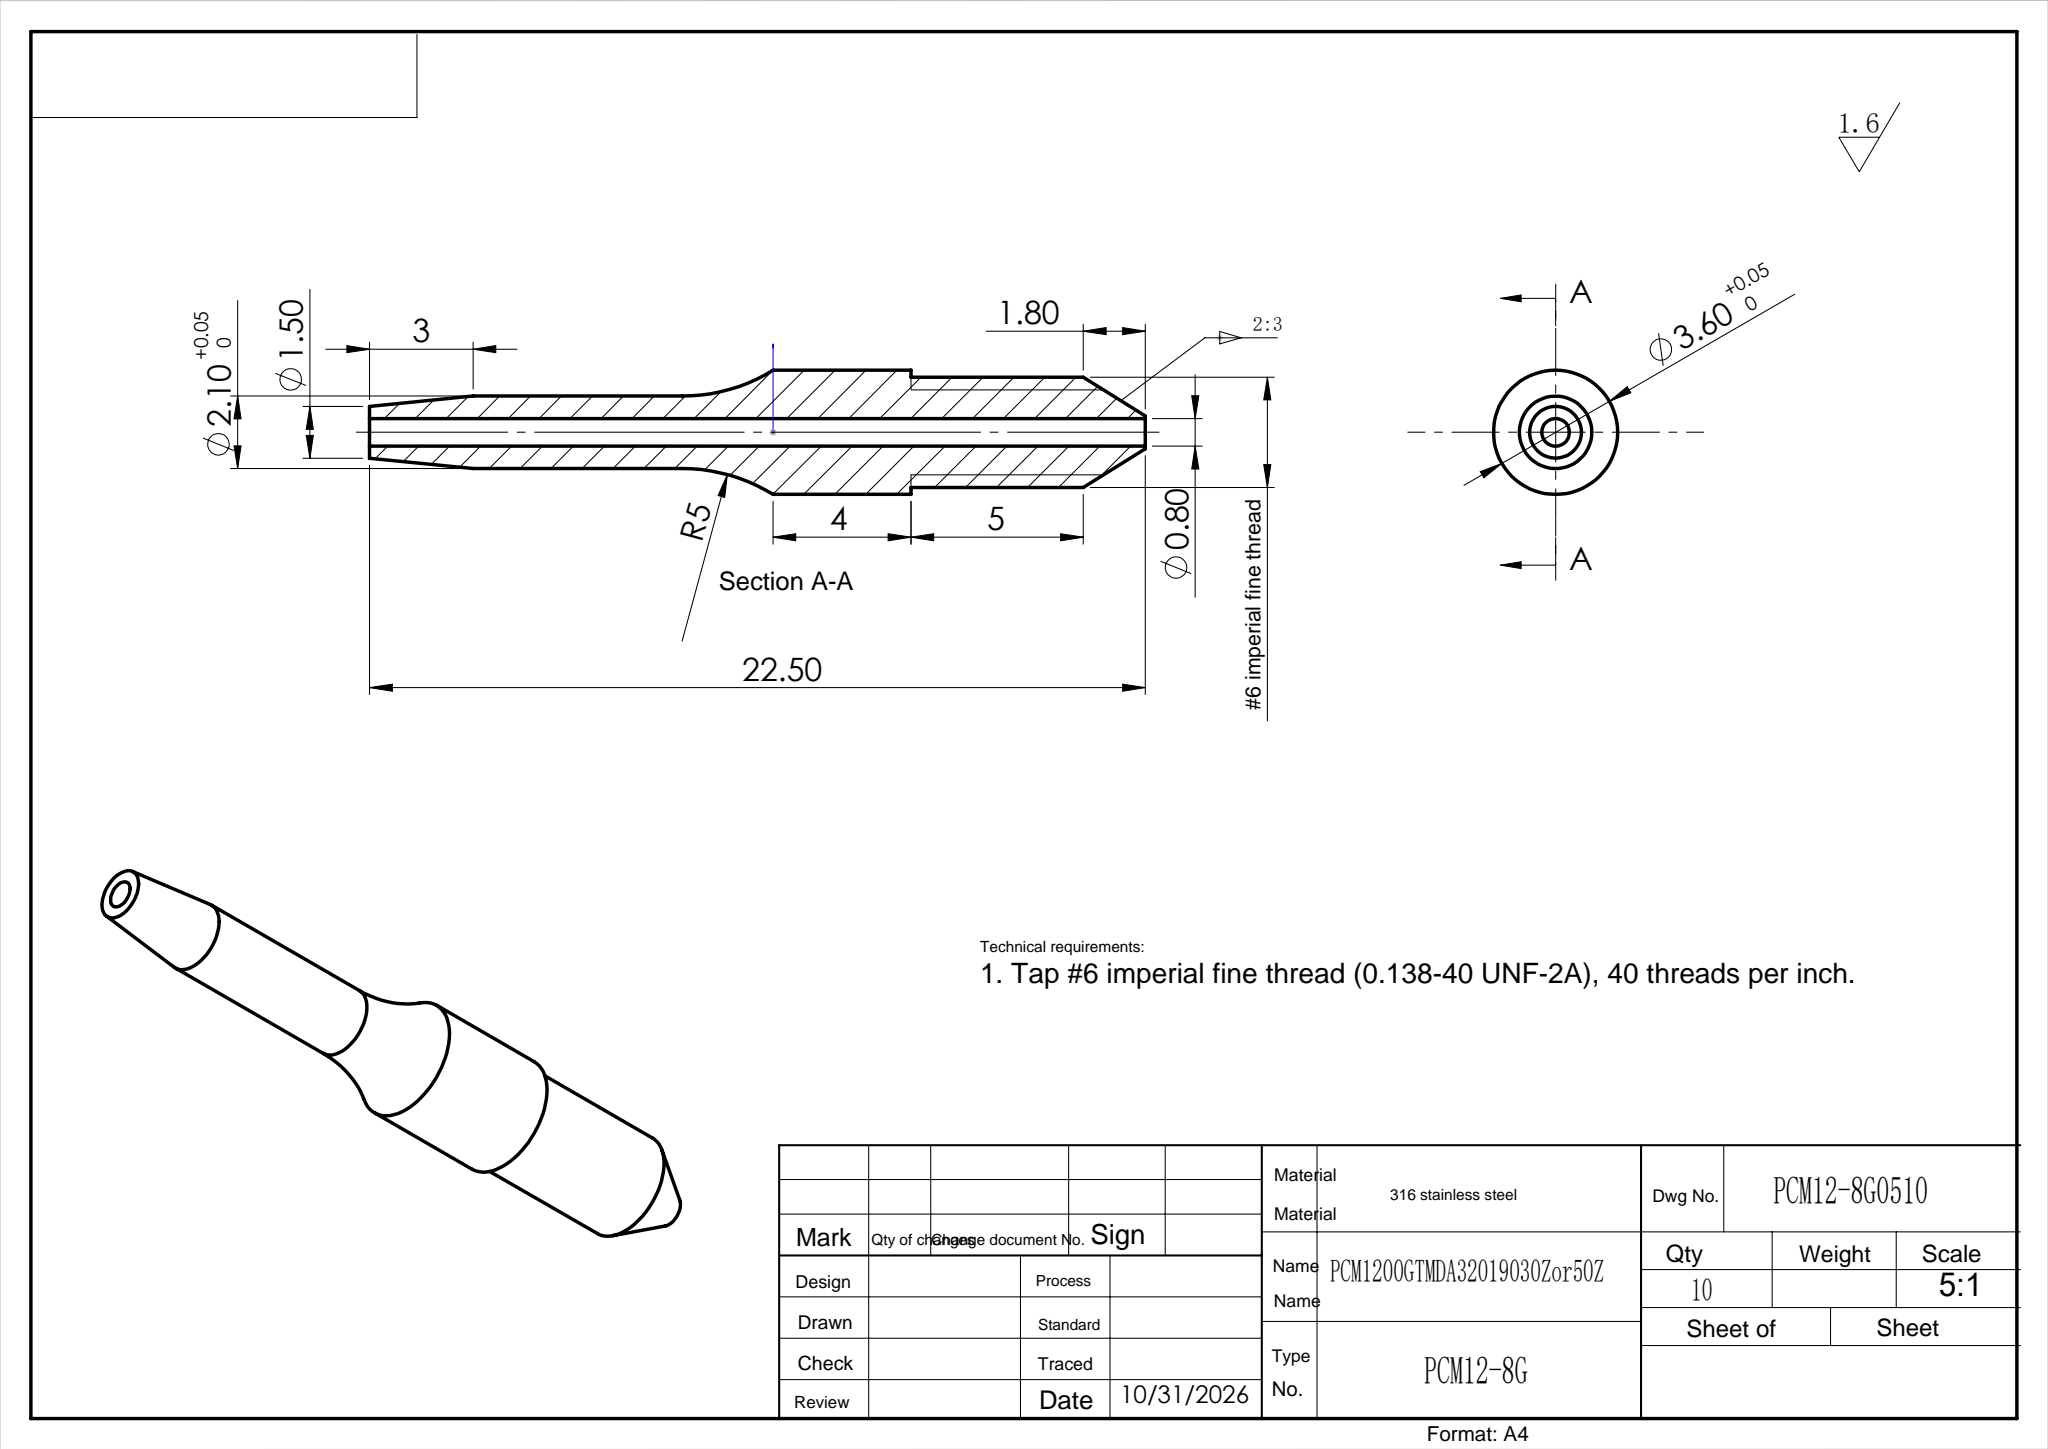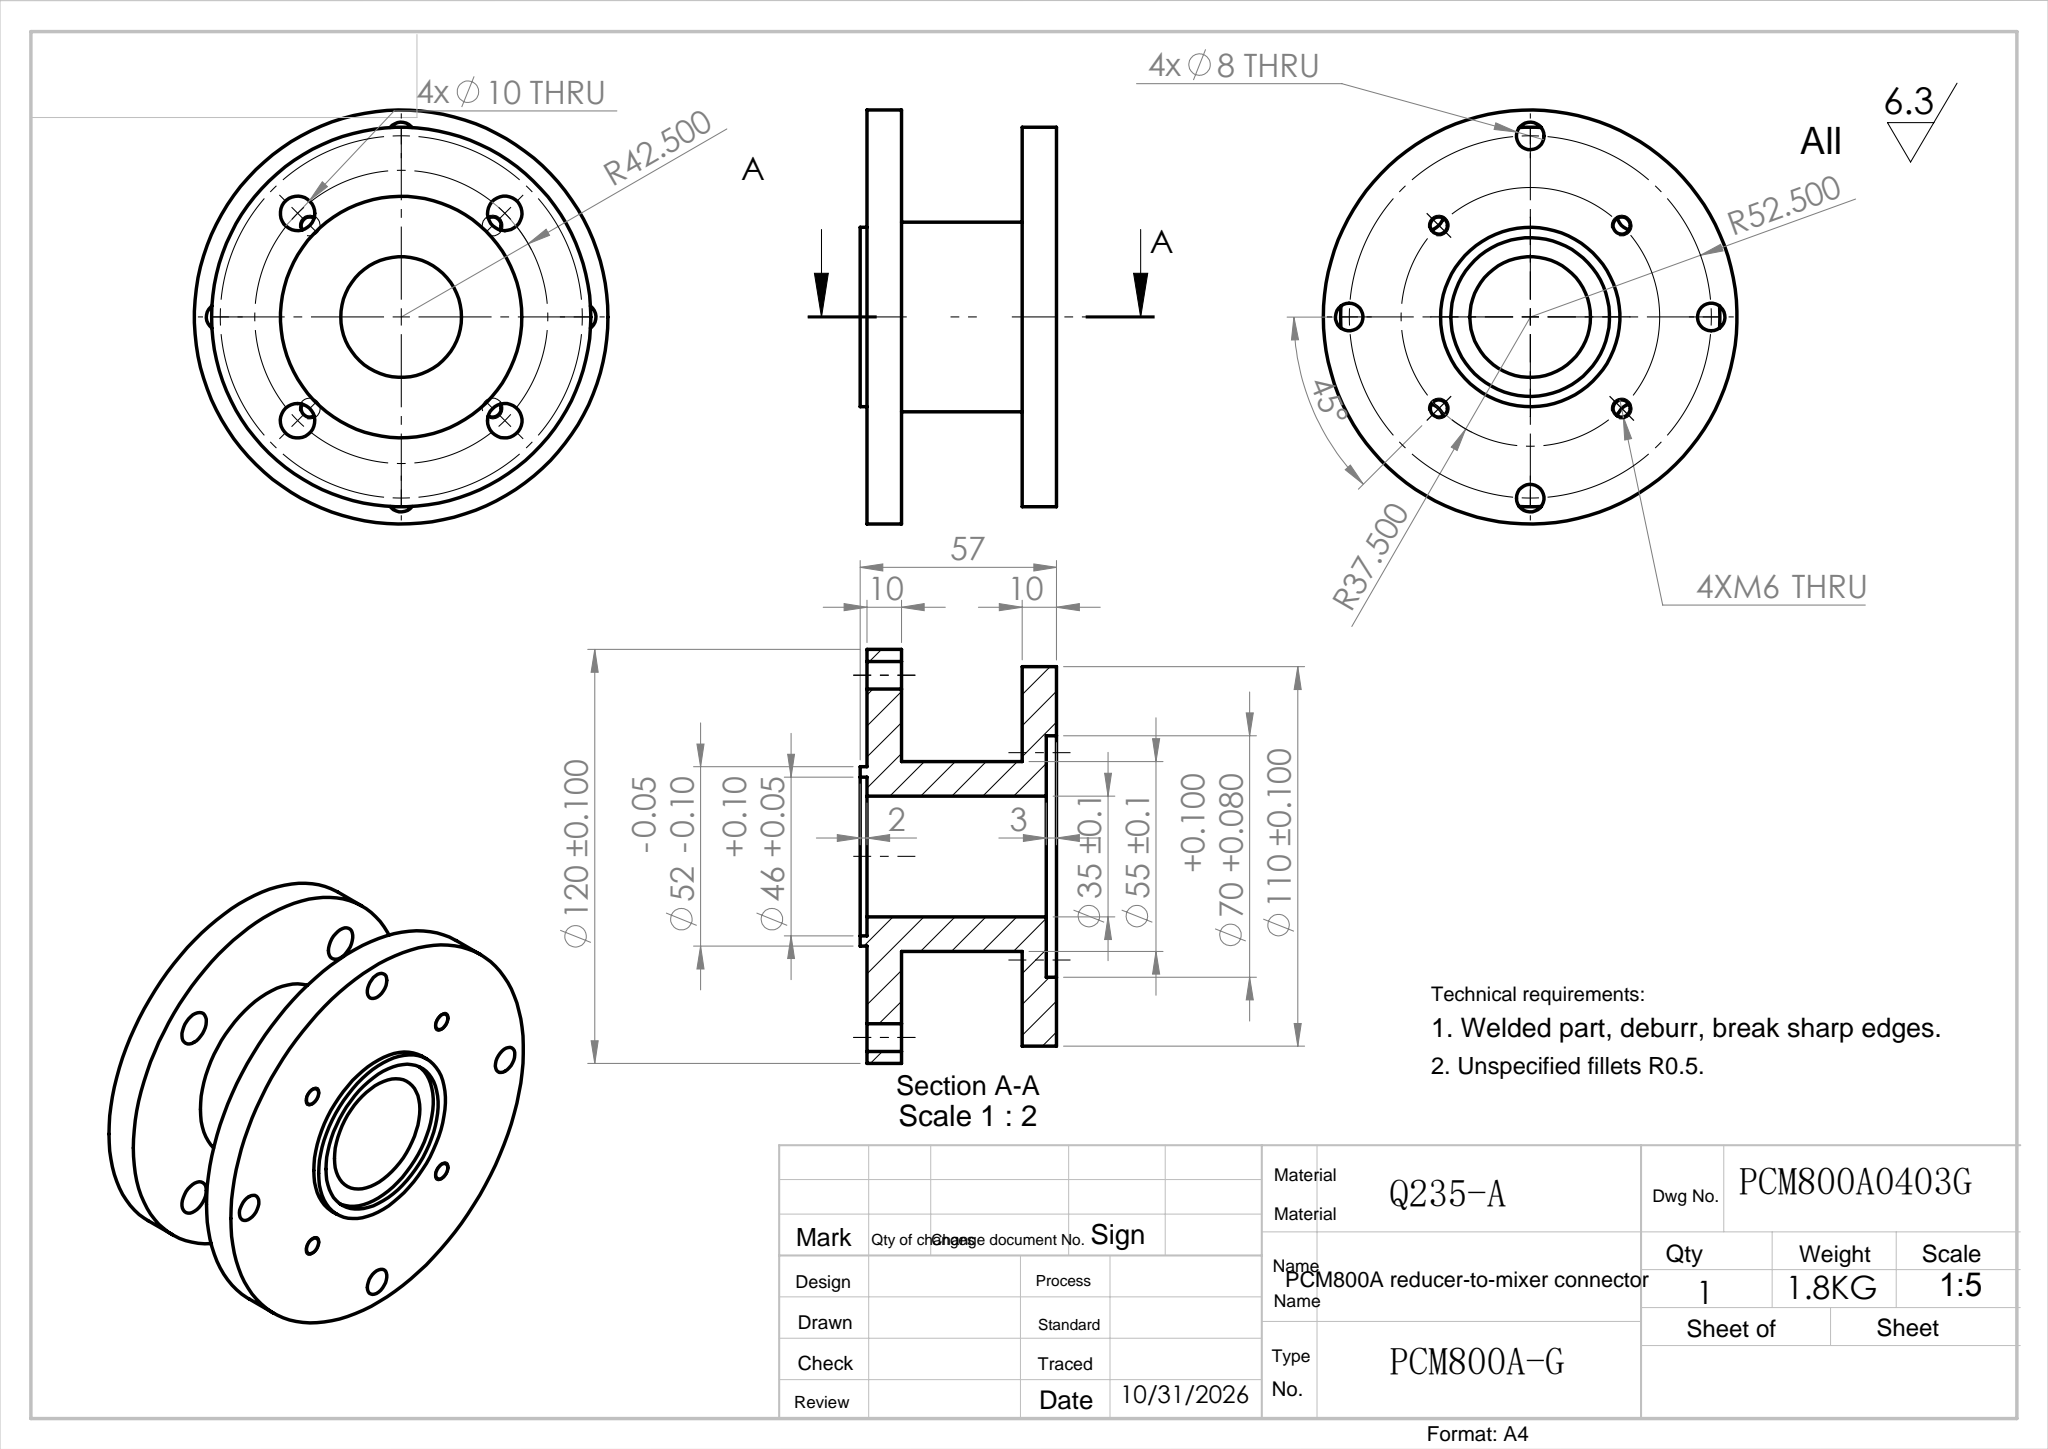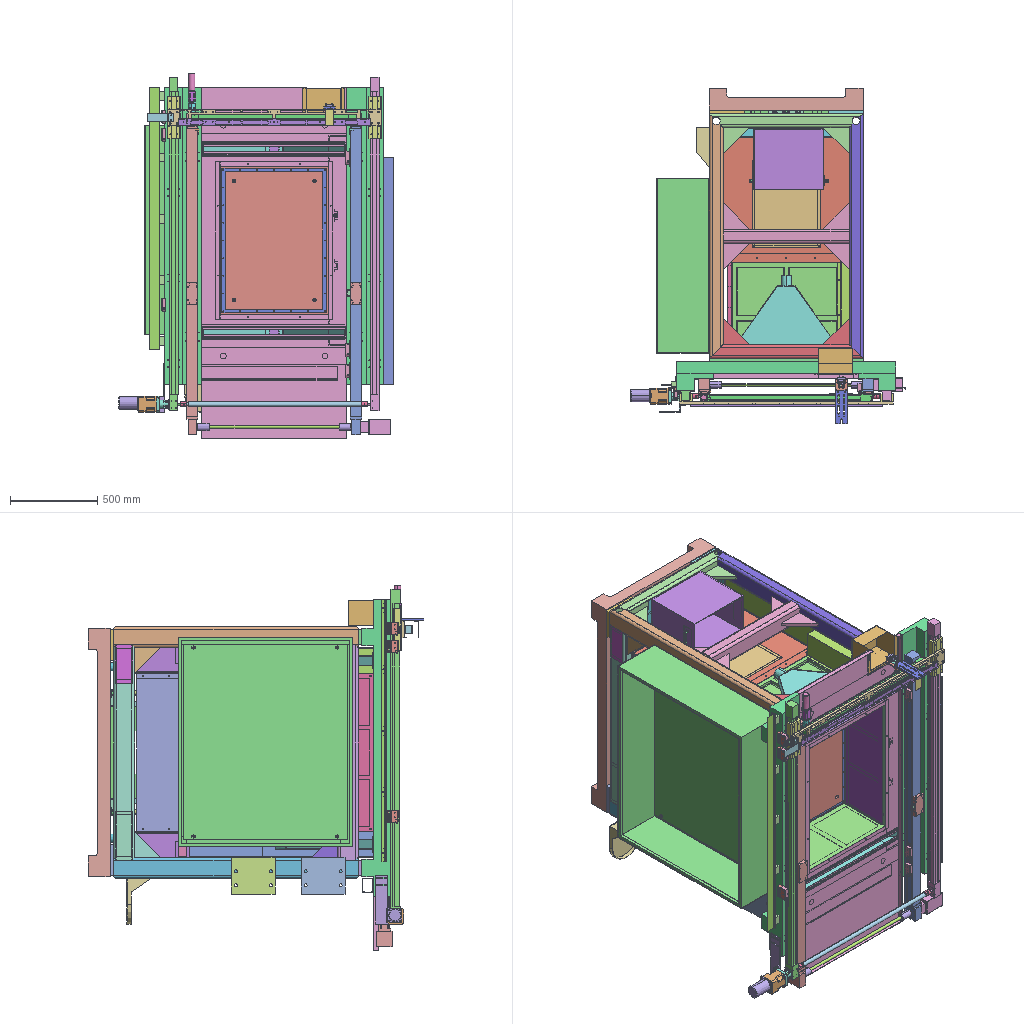Assembly | SolidWorks | 213 different items | 390 placed | box 1571 x 1918 x 2089 mm
Parts list (item | name | quantity | parent item | size | volume | features):
1 | (subassembly) | x1 | in 20 | 45.671 x 31.209 x 79.324 mm | 36091 mm3 | -
2 | (subassembly) | x2 | in 1 | 11.2 x 79.113 x 5.6 mm | 906.583 mm3 | features CompositeCurve 1
3 | (subassembly) | x1 | in 20 | 158.75 x 253.079 x 184.571 mm | 227945 mm3 | -
4 | (subassembly) | x2 | in 6 | 450 x 350 x 250 mm | 2820249 mm3 | features AEMSimFeature 1
5 | (subassembly) | x2 | in 8 | 202.5 x 1859 x 119.5 mm | 4220516 mm3 | features CompositeCurve 1
6 | (subassembly) | x1 | - | 1731 x 1422 x 2008 mm | 170873319 mm3 | features CompositeCurve 1
7 | (subassembly) | x1 | - | - | 100167004 mm3 | features ReferencePattern 16, CompositeCurve 9, LocalLPattern 2
8 | (subassembly) | x1 | - | - | 140729091 mm3 | features CompositeCurve 2
9 | (subassembly) | x2 | in 7 | 121 x 153.5 x 29.5 mm | 51392 mm3 | -
10 | (subassembly) | x2 | in 7 | 52.5 x 15 x 65 mm | 16522 mm3 | -
11 | (subassembly) | x1 | in 7 | 103 x 363 x 86 mm | 1173870 mm3 | -
12 | (subassembly) | x1 | in 7 | 64.002 x 64.002 x 160 mm | 203839 mm3 | -
13 | (subassembly) | x1 | in 7 | 45.805 x 40.368 x 35 mm | 17683 mm3 | -
14 | (subassembly) | x3 | - | 26 x 65 x 74.506 mm | 84061 mm3 | -
15 | (subassembly) | x3 | - | 100 x 42 x 26 mm | 68056 mm3 | -
16 | (subassembly) | x2 | in 7 | 120 x 42 x 41 mm | 79565 mm3 | -
17 | (subassembly) | x1 | in 8 | 700 x 1398 x 750 mm | 37335831 mm3 | features AEMSimFeature 1
18 | (subassembly) | x1 | - | 1167 x 88 x 1837 mm | 15808728 mm3 | -
19 | (subassembly) | x1 | in 17 | 472.19 x 352.538 x 235.211 mm | 7182982 mm3 | features AEMSimFeature 1
20 | (subassembly) | x1 | - | 300.5 x 279.222 x 1337 mm | 3097922 mm3 | features CompositeCurve 1
21 | (subassembly) | x1 | - | 2273 x 1295 x 1895 mm | 10477975 mm3 | -
22 | - | x1 | in 8 | 782 x 83 x 1038 mm | 2557655 mm3 | features ICE 6, Extrusion 1, Shell 1
23 | - | x2 | in 2 | 3.4 x 3.4 x 17.8 mm | 96.571 mm3 | features Boss 2, Chamfer 1, Cut 1, Extrusion 1, Fillet 1
24 | - | x2 | in 2 | 3.6 x 3.6 x 17.8 mm | 95.144 mm3 | features Chamfer 3, Boss 2, Extrusion 1
25 | - | x2 | in 2 | 5.6 x 11.2 x 40 mm | 624.39 mm3 | features Boss 6, Cut 3, Fillet 3, MirrorPattern 3, Chamfer 1, Extrusion 1, Sweep 1
26 | - | x1 | in 1 | 15 x 18 x 30 mm | 6618 mm3 | features Cut 3, Extrusion 1, LPattern 1
27 | - | x1 | in 1 | 12.5 x 8 x 8.081 mm | 341.66 mm3 | features Boss 1, Cut 1, Extrusion 1
28 | - | x1 | in 1 | 35 x 24 x 45 mm | 15822 mm3 | features Cut 6, Boss 2, MirrorPattern 2, Extrusion 1, Fillet 1
29 | - | x1 | in 1 | 55 x 12.5 x 40 mm | 11308 mm3 | features Boss 3, Cut 3, Extrusion 1, Fillet 1, HoleWzd 1, ICE 1, MirrorPattern 1
30 | - | x1 | in 3 | 72 x 66 x 80 mm | 80733 mm3 | features Boss 3, HoleWzd 3, Extrusion 1, MirrorPattern 1
31 | - | x1 | in 3 | 66 x 10 x 190 mm | 102125 mm3 | features Cut 2, HoleWzd 2, Extrusion 1
32 | - | x1 | in 3 | 51 x 261 x 69 mm | 43977 mm3 | features Extrusion 1, ICE 1, LPattern 1, Shell 1
33 | - | x1 | in 8 | 841 x 100 x 1142 mm | 2713356 mm3 | features ICE 5, Extrusion 1, Shell 1
34 | - | x2 | in 2 | 3 x 3 x 20 mm | 90.478 mm3 | features Extrusion 1
35 | - | x1 | in 6 | 280 x 70 x 48.5 mm | 177998 mm3 | features Extrusion 1, HoleWzd 1, ICE 1
36 | - | x1 | in 6 | 78.5 x 60 x 800 mm | 272371 mm3 | features ExtruThin 1, HoleWzd 1, MirrorPattern 1
37 | - | x1 | in 6 | 8 x 63 x 800 mm | 91142 mm3 | features ExtruThin 1, HoleWzd 1, MirrorPattern 1
38 | - | x1 | in 6 | 238 x 166 x 150 mm | 256776 mm3 | features ICE 2, Extrusion 1, Shell 1
39 | - | x2 | in 6 | 822.906 x 560 x 70 mm | 1097243 mm3 | features ICE 2, Extrusion 1, Shell 1
40 | - | x2 | in 4 | 410 x 350 x 250 mm | 2798000 mm3 | features ICE 2, Extrusion 1, Shell 1
41 | - | x4 | in 4 | 120 x 20 x 15 mm | 11124 mm3 | features Extrusion 1, Fillet 1, ICE 1
42 | - | x2 | in 6 | 715 x 153 x 250 mm | 795621 mm3 | features ICE 5, Extrusion 1
43 | - | x1 | in 8 | 295 x 2005 x 250 mm | 2083546 mm3 | features ICE 7, Extrusion 1, Shell 1
44 | - | x2 | in 5 | 202.5 x 359 x 119.5 mm | 3868562 mm3 | features ICE 6, Extrusion 1
45 | - | x1 | in 6 | 880 x 125 x 1420 mm | 55146557 mm3 | features Fillet 3, 3DProfileFeature 2, Cut 2, HoleWzd 2, LPattern 2, Extrusion 1, ICE 1
46 | - | x1 | in 6 | 220 x 100 x 1 mm | 22000 mm3 | features Extrusion 1
47 | - | x1 | in 6 | 280 x 100 x 1 mm | 28000 mm3 | features Extrusion 1
48 | - | x1 | in 6 | 60 x 60 x 1 mm | 2477 mm3 | features Extrusion 1
49 | - | x1 | in 6 | 55 x 11 x 55 mm | 19851 mm3 | features Revolution 1
50 | - | x1 | - | 146 x 1366 x 130.5 mm | 474775 mm3 | features ICE 8, HoleWzd 2, Extrusion 1
51 | - | x1 | in 8 | 150 x 480 x 2005 mm | 2840339 mm3 | features ICE 8, ExtruThin 1
52 | - | x1 | - | 146 x 1366 x 130.5 mm | 474775 mm3 | features ICE 8, HoleWzd 2, Extrusion 1
53 | - | x1 | in 6 | 1438 x 898.415 x 1530 mm | 49681845 mm3 | features ICE 6, Boss 5, MirrorPattern 4, WeldMemberFeat 3, HoleWzd 2, LPattern 2, MirrorSolid 2, 3DProfileFeature 1, Cut 1, WeldmentFeature 1
54 | - | x1 | in 6 | 120 x 60 x 50 mm | 42021 mm3 | features ExtruThin 1, ICE 1
55 | - | x1 | in 6 | 1200 x 1000 x 300 mm | 7626457 mm3 | features ICE 7, LPattern 3, Extrusion 1, Fillet 1, Shell 1
56 | - | x1 | in 6 | 230 x 250 x 265 mm | 373785 mm3 | features ICE 4, Rib 2, Extrusion 1
57 | - | x1 | in 6 | 830 x 2008 x 32.5 mm | 2572177 mm3 | features ICE 8, Extrusion 1, LPattern 1
58 | - | x1 | in 6 | 1252 x 168 x 1700 mm | 44599924 mm3 | features ICE 4, HoleWzd 3, Fillet 2, Shell 2, Extrusion 1, MirrorPattern 1
59 | - | x2 | in 5 | 76 x 76 x 1500 mm | 351954 mm3 | features Extrusion 1, ICE 1
60 | - | x1 | in 8 | 787 x 165 x 100 mm | 713791 mm3 | features ICE 2, Extrusion 1, Shell 1
61 | - | x4 | in 7 | 110 x 10 x 110 mm | 48026 mm3 | features HoleWzd 1, Revolution 1
62 | - | x2 | in 7 | 623 x 635 x 25 mm | 3690263 mm3 | features Boss 8, Cut 3, 3DProfileFeature 2, HoleWzd 2, Chamfer 1, Extrusion 1, Fillet 1
63 | - | x2 | in 7 | 25 x 635 x 2 mm | 31411 mm3 | features Cut 1, Extrusion 1, LPattern 1
64 | - | x2 | in 7 | 47 x 14 x 47 mm | 19838 mm3 | features Chamfer 1, Extrusion 1
65 | - | x2 | in 7 | 110 x 110 x 24 mm | 185226 mm3 | features Cut 3, 3DProfileFeature 2, Chamfer 2, HoleWzd 2, Extrusion 1, Fillet 1
66 | - | x2 | in 7 | 75 x 10 x 75 mm | 20954 mm3 | features Chamfer 2, Boss 1, Cut 1, Extrusion 1, Fillet 1
67 | - | x8 | in 7 | 23 x 115 x 10 mm | 9831 mm3 | features Extrusion 1, ICE 1
68 | - | x2 | in 7 | 47 x 44 x 47 mm | 38423 mm3 | features Boss 2, Chamfer 1, Cut 1, Extrusion 1
69 | - | x2 | in 7 | 200 x 79 x 115 mm | 1064261 mm3 | features Cut 7, Boss 2, HoleWzd 2, ICE 2, Extrusion 1, Fillet 1, MirrorPattern 1
70 | - | x2 | in 7 | 186.408 x 27 x 186.408 mm | 546884 mm3 | features Cut 5, Chamfer 3, Extrusion 1
71 | - | x1 | in 8 | 1204 x 492 x 30 mm | 1446455 mm3 | features ICE 3, Extrusion 1, Shell 1
72 | - | x4 | in 7 | 760 x 29 x 34 mm | 720073 mm3 | features Cut 2, Extrusion 1, LPattern 1
73 | - | x20 | in 7 | 23 x 20 x 9 mm | 3318 mm3 | features Cut 2, Extrusion 1
74 | - | x4 | in 7 | 135 x 40.5 x 70 mm | 280823 mm3 | features Cut 2, Extrusion 1
75 | - | x4 | in 7 | 50 x 50 x 835 mm | 1540803 mm3 | features Boss 2, Extrusion 1, HoleWzd 1, ICE 1, RevCut 1
76 | - | x8 | in 7 | 49.742 x 49.742 x 8 mm | 7088 mm3 | features Extrusion 1
77 | - | x1 | in 7 | 740 x 870 x 540 mm | 47222068 mm3 | features HoleWzd 9, 3DProfileFeature 8, MirrorPattern 7, Cut 5, Fillet 5, Boss 2, LPattern 2, Extrusion 1
78 | - | x3 | in 7 | 10.158 x 8.5 x 585 mm | 43311 mm3 | features Extrusion 1
79 | - | x2 | in 7 | 25 x 834 x 25 mm | 365070 mm3 | features Boss 4, Fillet 2, Chamfer 1, Extrusion 1
80 | - | x2 | in 7 | 48 x 81 x 62 mm | 73064 mm3 | features Boss 2, Cut 2, Chamfer 1, Extrusion 1
81 | - | x2 | in 7 | 520 x 100 x 100 mm | 2650054 mm3 | features Cut 5, Attribute 4, ICE 3, Extrusion 1, Fillet 1, HoleWzd 1, MirrorPattern 1
82 | - | x1 | in 8 | 1204 x 230 x 30 mm | 710869 mm3 | features ICE 3, Extrusion 1, Shell 1
83 | - | x4 | in 7 | 47 x 15 x 47 mm | 22564 mm3 | features Extrusion 1, Fillet 1
84 | - | x2 | in 7 | 80 x 80 x 17 mm | 23688 mm3 | features Boss 2, Chamfer 1, Cut 1, Extrusion 1, Fillet 1
85 | - | x2 | in 7 | 28 x 16 x 28 mm | 5744 mm3 | features Chamfer 1, Extrusion 1
86 | - | x2 | in 7 | 37 x 18 x 37 mm | 13677 mm3 | features Fillet 3, HoleWzd 3, 3DProfileFeature 2, Boss 1, CirPattern 1, Cut 1, Extrusion 1, ICE 1
87 | - | x2 | in 7 | 90 x 75 x 12 mm | 42464 mm3 | features Cut 2, Boss 1, Extrusion 1
88 | - | x1 | in 7 | 900 x 760 x 50 mm | 1252591 mm3 | features ICE 4, Cut 2, HoleWzd 2, Extrusion 1, Fillet 1, MirrorPattern 1, Shell 1
89 | - | x2 | in 7 | 390 x 500 x 1 mm | 194905 mm3 | features Extrusion 1, ICE 1
90 | - | x2 | in 7 | 760 x 720 x 30 mm | 624524 mm3 | features ICE 7, Fillet 2, Extrusion 1, HoleWzd 1
91 | - | x2 | in 7 | 903 x 720 x 1 mm | 649804 mm3 | features Extrusion 1, ICE 1
92 | - | x1 | in 7 | 827 x 5 x 597 mm | 274573 mm3 | features LPattern 3, Cut 1, Extrusion 1
93 | - | x2 | in 8 | 598.5 x 1319 x 28 mm | 1912739 mm3 | features Extrusion 1, ICE 1, Shell 1
94 | - | x1 | in 7 | 60 x 635 x 900 mm | 5489881 mm3 | features Boss 5, 3DProfileFeature 2, HoleWzd 2, Extrusion 1, MirrorPattern 1
95 | - | x1 | in 7 | 60 x 25 x 900 mm | 665333 mm3 | features 3DProfileFeature 3, HoleWzd 3, Boss 1, Chamfer 1, Cut 1, Extrusion 1, LPattern 1
96 | - | x1 | in 7 | 25 x 900 x 25 mm | 491836 mm3 | features 3DProfileFeature 2, HoleWzd 2, Chamfer 1, Cut 1, Extrusion 1, LPattern 1
97 | - | x1 | in 7 | 25 x 583 x 900 mm | 4907028 mm3 | features Boss 4, 3DProfileFeature 3, HoleWzd 3, LPattern 3, Chamfer 2, Cut 2, Extrusion 1
98 | - | x2 | in 9 | 95 x 20 x 120 mm | 16175 mm3 | features ICE 2, Chamfer 1, Extrusion 1
99 | - | x2 | in 9 | 72 x 29.5 x 20 mm | 17819 mm3 | features Extrusion 1, Fillet 1, ICE 1
100 | - | x2 | in 7 | 200 x 55 x 20 mm | 28430 mm3 | features ExtruThin 1, ICE 1
101 | - | x2 | in 10 | 35 x 65 x 10 mm | 6719 mm3 | features Fillet 1, Sweep 1
102 | - | x2 | in 9 | 70 x 130 x 23.5 mm | 17397 mm3 | features ICE 2, Extrusion 1, LPattern 1
103 | - | x4 | in 10 | 45 x 13 x 20 mm | 4902 mm3 | features Extrusion 1, Fillet 1, ICE 1
104 | - | x1 | in 8 | 1210 x 260 x 30 mm | 849119 mm3 | features ICE 3, Extrusion 1, Shell 1
105 | - | x1 | in 7 | 617 x 20 x 847 mm | 9301034 mm3 | features LPattern 3, Cut 2, HoleWzd 2, ICE 2, 3DProfileFeature 1, Extrusion 1
106 | - | x1 | in 7 | 10.158 x 8.5 x 900 mm | 66632 mm3 | features Extrusion 1
107 | - | x1 | in 11 | 124 x 13 x 13 mm | 14963 mm3 | features Boss 6, Fillet 3, Chamfer 1, Cut 1
108 | - | x1 | in 11 | 102.5 x 50 x 85 mm | 153933 mm3 | features Cut 3, 3DProfileFeature 1, Boss 1, Extrusion 1, HoleWzd 1, Split 1, WeldBeadFeat 1, WeldmentFeature 1
109 | - | x1 | in 11 | 80 x 80 x 184 mm | 810663 mm3 | features ICE 6, CombineBodies 1, Extrusion 1, Fillet 1
110 | - | x1 | in 11 | 103 x 53 x 86 mm | 69237 mm3 | features HoleWzd 2, 3DProfileFeature 1, Boss 1, Extrusion 1, ICE 1, Split 1, WeldBeadFeat 1, WeldmentFeature 1
111 | - | x1 | in 11 | 50 x 78 x 38 mm | 42138 mm3 | features Cut 3, Chamfer 2, Gusset 2, WeldBeadFeat 2, Boss 1, Extrusion 1, Fillet 1, WeldmentFeature 1
112 | - | x1 | in 8 | 1210 x 230 x 30 mm | 714301 mm3 | features ICE 3, Extrusion 1, Shell 1
113 | - | x1 | in 11 | 38 x 30 x 38 mm | 16522 mm3 | features Boss 2, Extrusion 1
114 | - | x1 | in 11 | 35.736 x 27 x 35.736 mm | 11879 mm3 | features Cut 2, Chamfer 1, Extrusion 1
115 | - | x1 | in 11 | 25 x 4 x 4 mm | 393.133 mm3 | features Extrusion 1
116 | - | x1 | in 11 | 40 x 40 x 66 mm | 50078 mm3 | features Cut 5, Boss 2, Chamfer 1, Extrusion 1
117 | - | x2 | in 11 | 24 x 6 x 24 mm | 2031 mm3 | features Chamfer 1, Extrusion 1
118 | - | x2 | in 12, 13 | 40 x 40 x 100 mm | 62655 mm3 | features Fillet 1, MirrorStock 1
119 | - | x1 | in 12 | 50 x 49 x 49 mm | 86970 mm3 | features HoleWzd 2, Extrusion 1, ICE 1
120 | - | x4 | in 12, 13 | 19 x 1.5 x 19 mm | 138.591 mm3 | features Extrusion 1
121 | - | x1 | in 13 | 50 x 49 x 49 mm | 86970 mm3 | features HoleWzd 2, Extrusion 1, ICE 1
122 | - | x4 | in 12, 13 | 35 x 11 x 35 mm | 8600 mm3 | features MirrorStock 1
123 | - | x2 | in 8 | 1346 x 22 x 288 mm | 1655952 mm3 | features ICE 2, Extrusion 1, Shell 1
124 | - | x1 | in 8 | 641 x 270 x 2005 mm | 4371242 mm3 | features ICE 11, ExtruThin 1
125 | - | x2 | in 12, 13 | 49 x 10 x 49 mm | 22243 mm3 | features 3DProfileFeature 1, Cut 1, Extrusion 1, HoleWzd 1
126 | - | x4 | in 12, 13 | 1 x 19.276 x 18.3 mm | 102.745 mm3 | features Boss 1, Cut 1, Extrusion 1
127 | - | x2 | in 12, 13 | 15 x 48 x 15 mm | 8443 mm3 | features MirrorStock 1
128 | - | x2 | in 12, 13 | 12 x 12 x 61 mm | 5846 mm3 | features ICE 3, Chamfer 2, MirrorStock 1
129 | - | x2 | in 7 | 70 x 30 x 10.5 mm | 20714 mm3 | features Extrusion 1
130 | - | x8 | in 14, 15, 16 | 74.506 x 42 x 21 mm | 49715 mm3 | features Extrusion 1, ICE 1
131 | - | x3 | in 15 | 100 x 37 x 5 mm | 18341 mm3 | features Extrusion 1, ICE 1
132 | - | x3 | in 14 | 20 x 60 x 70 mm | 34346 mm3 | features ICE 2, Extrusion 1
133 | - | x2 | in 16 | 120 x 37 x 5 mm | 21137 mm3 | features Extrusion 1
134 | - | x4 | in 16 | 20 x 20 x 15 mm | 4356 mm3 | features Extrusion 1
135 | - | x1 | in 8 | 370 x 270 x 2005 mm | 2609209 mm3 | features ICE 10, ExtruThin 1
136 | - | x2 | - | 40 x 25 x 12 mm | 6861 mm3 | features ICE 2, Extrusion 1, Fillet 1
137 | - | x1 | in 7 | 70 x 36 x 15 mm | 19658 mm3 | features Extrusion 1, Fillet 1, HoleWzd 1
138 | - | x2 | in 8 | 601 x 1551 x 28 mm | 2239470 mm3 | features Extrusion 1, ICE 1, Shell 1
139 | - | x1 | in 8 | 645 x 596 x 22 mm | 953984 mm3 | features Extrusion 1, ICE 1, Shell 1
140 | - | x1 | in 8 | 1457 x 492 x 30 mm | 1732596 mm3 | features ICE 3, Extrusion 1, Shell 1
141 | - | x2 | - | 128 x 64 x 20 mm | 161397 mm3 | features HoleWzd 2, MirrorPattern 2, Extrusion 1, LPattern 1
142 | - | x1 | in 18 | 72 x 88 x 1836 mm | 7220915 mm3 | features Boss 5, Cut 2, Extrusion 1, MirrorPattern 1
143 | - | x1 | in 8 | 1457 x 230 x 30 mm | 855585 mm3 | features ICE 3, Extrusion 1, Shell 1
144 | - | x1 | in 18 | 80 x 88 x 1836 mm | 7212179 mm3 | features Boss 5, Cut 2, MirrorPattern 2, Extrusion 1
145 | - | x1 | in 18 | 90 x 80 x 175 mm | 1069126 mm3 | features Boss 1, Chamfer 1, Cut 1, Extrusion 1
146 | - | x1 | in 18 | 16 x 16 x 770 mm | 154818 mm3 | features Extrusion 1
147 | - | x1 | in 6 | 55.5 x 21 x 1300 mm | 146072 mm3 | features ExtruThin 1, ICE 1
148 | - | x2 | in 18 | 40 x 40 x 67 mm | 70724 mm3 | features Extrusion 1, ICE 1
149 | - | x1 | in 18 | 35 x 32 x 20 mm | 5122 mm3 | features ICE 2, Extrusion 1
150 | - | x1 | in 18 | 35 x 32 x 20 mm | 5122 mm3 | features ICE 2, Extrusion 1
151 | - | x2 | in 8 | 724.5 x 1319 x 28 mm | 2267303 mm3 | features Extrusion 1, ICE 1, Shell 1
152 | - | x1 | in 8 | 2010 x 1894 x 432 mm | 6181114 mm3 | features ICE 6, WeldMemberFeat 3, WeldmentFeature 1
153 | - | x1 | in 8 | 2010 x 1894 x 230 mm | 4743265 mm3 | features ICE 6, WeldMemberFeat 3, WeldmentFeature 1
154 | - | x1 | in 8 | 841 x 100 x 658 mm | 1673891 mm3 | features ICE 5, Extrusion 1, Shell 1
155 | - | x1 | in 8 | 1740 x 2160 x 55 mm | 4890635 mm3 | features ICE 7, WeldMemberFeat 1, WeldmentFeature 1
156 | - | x1 | in 8 | 745 x 1196 x 22 mm | 2073584 mm3 | features Extrusion 1, ICE 1, Shell 1
157 | - | x1 | in 8 | 980 x 650 x 1400 mm | 5357860 mm3 | features ICE 6, Extrusion 1
158 | - | x1 | in 8 | 980 x 100 x 1400 mm | 3675222 mm3 | features ICE 8, Extrusion 1, HoleWzd 1, Shell 1
159 | - | x2 | in 3 | 21 x 8.5 x 8.5 mm | 554.946 mm3 | features Fillet 2, RevCut 2, Attribute 1, Cut 1, LPattern 1, Revolution 1
160 | - | x2 | in 1 | 9.8 x 5.6 x 5.6 mm | 93.48 mm3 | features Fillet 2, Attribute 1, Cut 1, LPattern 1, RevCut 1, Revolution 1
161 | - | x1 | in 8 | 980 x 100 x 1400 mm | 2213321 mm3 | features ICE 10, Extrusion 1
162 | - | x1 | in 8 | 367 x 646 x 20 mm | 519095 mm3 | features ICE 2, Extrusion 1, Shell 1
163 | - | x1 | in 8 | 609 x 323 x 20 mm | 403774 mm3 | features ICE 3, Extrusion 1, Shell 1
164 | - | x1 | in 8 | 609 x 323 x 20 mm | 440064 mm3 | features ICE 3, Extrusion 1, Shell 1
165 | - | x1 | in 8 | 850 x 400 x 770 mm | 3305317 mm3 | features ICE 9, Extrusion 1, HoleWzd 1, Shell 1
166 | - | x1 | in 8 | 1750 x 200 x 1290 mm | 4398442 mm3 | features ICE 16, MirrorPattern 2, Extrusion 1, HoleWzd 1
167 | - | x1 | in 8 | 1600 x 167 x 205 mm | 1759661 mm3 | features ICE 5, Extrusion 1, Shell 1
168 | - | x1 | in 8 | 2015 x 437 x 116 mm | 1908304 mm3 | features ICE 7, Extrusion 1
169 | - | x2 | in 8 | 117 x 1256 x 128 mm | 462770 mm3 | features ICE 4, Extrusion 1
170 | - | x2 | in 8 | 180 x 156 x 120 mm | 128045 mm3 | features ICE 3, Extrusion 1
171 | - | x16 | in 8 | 23.5 x 55 x 8.5 mm | 8792 mm3 | features Extrusion 1, ICE 1
172 | - | x16 | in 8 | 23.5 x 55 x 8.5 mm | 8792 mm3 | features Extrusion 1, ICE 1
173 | - | x1 | in 17 | 600 x 5 x 700 mm | 2085945 mm3 | features Extrusion 1, ICE 1
174 | - | x1 | in 17 | 700 x 750 x 40 mm | 20800000 mm3 | features Extrusion 1
175 | - | x1 | in 19 | 35 x 315 x 50 mm | 548501 mm3 | features Extrusion 1, ICE 1
176 | - | x1 | in 19 | 440 x 60 x 292 mm | 6071392 mm3 | features ICE 3, Extrusion 1
177 | - | x1 | in 19 | 148.985 x 148.985 x 26.5 mm | 50583 mm3 | features ICE 3, Extrusion 1, RefAxis 1, RevCut 1
178 | - | x1 | in 19 | 130 x 80 x 125 mm | 284219 mm3 | features ICE 3, Extrusion 1
179 | - | x1 | in 8 | 2015 x 235 x 116 mm | 1204410 mm3 | features ICE 6, Extrusion 1
180 | - | x2 | in 19 | 45 x 45 x 90 mm | 73587 mm3 | features ICE 5, Extrusion 1
181 | - | x1 | in 19 | 35 x 40 x 187.5 mm | 57604 mm3 | features ICE 3, Extrusion 1
182 | - | x1 | in 19 | 30 x 35 x 30 mm | 12087 mm3 | features ICE 4, Extrusion 1
183 | - | x1 | in 19 | 20 x 23 x 30 mm | 11422 mm3 | features ICE 3, Extrusion 1
184 | - | x1 | in 17 | 400 x 30 x 800 mm | 1395984 mm3 | features ICE 2, Extrusion 1, Shell 1
185 | - | x1 | in 17 | 600 x 125 x 1000 mm | 1467494 mm3 | features ICE 11, Extrusion 1, Shell 1
186 | - | x1 | in 17 | 600 x 1000 x 425 mm | 2418347 mm3 | features ICE 5, Extrusion 1, Shell 1
187 | - | x1 | in 17 | 600 x 1000 x 150 mm | 1985083 mm3 | features ICE 7, Extrusion 1, Shell 1
188 | - | x1 | in 8 | 1148 x 195 x 15 mm | 541900 mm3 | features ICE 2, Extrusion 1, Shell 1
189 | - | x1 | in 8 | 1148 x 125 x 15 mm | 375860 mm3 | features ICE 2, Extrusion 1, Shell 1
190 | - | x1 | in 20 | 44 x 12 x 1100 mm | 140604 mm3 | features Extrusion 1, ICE 1, LPattern 1
191 | - | x1 | in 20 | 95 x 25 x 50 mm | 17455 mm3 | features ExtruThin 1, ICE 1
192 | - | x1 | in 20 | 42 x 42 x 86.5 mm | 103966 mm3 | features Boss 5, Cut 4, Chamfer 2, Extrusion 1
193 | - | x1 | in 8 | 1750 x 167 x 200 mm | 1937226 mm3 | features ICE 5, HoleWzd 2, Extrusion 1, Shell 1
194 | - | x1 | in 20 | 64.5 x 44.058 x 985 mm | 1412008 mm3 | features Cut 3, Boss 2, Fillet 2, ICE 2, Chamfer 1, Extrusion 1, HoleWzd 1
195 | - | x1 | in 20 | 40 x 11 x 132 mm | 53803 mm3 | features Boss 2, Cut 2, Extrusion 1
196 | - | x1 | in 20 | 44 x 44 x 66.5 mm | 32907 mm3 | features Cut 7, Boss 3, 3DProfileFeature 1, Extrusion 1, HoleWzd 1
197 | - | x1 | in 20 | 95 x 16 x 1222 mm | 948675 mm3 | features HoleWzd 3, 3DProfileFeature 2, LPattern 2, Extrusion 1, Fillet 1, ICE 1
198 | - | x1 | in 20 | 38 x 38 x 128 mm | 121184 mm3 | features Boss 3, Chamfer 1, Cut 1, Extrusion 1
199 | - | x5 | in 6 | 50 x 25 x 30 mm | 36787 mm3 | features Extrusion 1, ICE 1
200 | - | x1 | in 6 | 1500 x 25 x 1 mm | 37381 mm3 | features Extrusion 1, ICE 1
201 | - | x1 | in 6 | 55.5 x 20 x 1500 mm | 166322 mm3 | features ExtruThin 1, ICE 1
202 | - | x2 | - | 76 x 44 x 240 mm | 396756 mm3 | features Cut 1, Extrusion 1
203 | - | x1 | in 20 | 150 x 45 x 50 mm | 47262 mm3 | features ExtruThin 1, ICE 1
204 | - | x1 | in 8 | 782 x 83 x 654 mm | 1247436 mm3 | features ICE 9, Extrusion 1, Shell 1
205 | - | x2 | in 21 | 30 x 30 x 35 mm | 19242 mm3 | features ICE 2, Extrusion 1
206 | - | x1 | in 21 | 25 x 25 x 1030 mm | 493959 mm3 | features ICE 2, Chamfer 1, Extrusion 1
207 | - | x1 | in 21 | 90 x 90 x 141 mm | 768294 mm3 | features Boss 4, Cut 3, Extrusion 1, Fillet 1
208 | - | x1 | in 21 | 74.5 x 55.5 x 1910 mm | 4257863 mm3 | features Boss 3, 3DProfileFeature 1, Chamfer 1, CirPattern 1, Cut 1, Extrusion 1, HoleWzd 1
209 | - | x1 | in 21 | 99 x 55.5 x 1910 mm | 4289434 mm3 | features Boss 3, 3DProfileFeature 1, Chamfer 1, CirPattern 1, Cut 1, Extrusion 1, HoleWzd 1, MirrorPattern 1
210 | - | x1 | in 21 | 80 x 80 x 149 mm | 513498 mm3 | features Boss 3, Chamfer 1, Cut 1, Extrusion 1
211 | - | x1 | in 21 | 90 x 90 x 77.5 mm | 116443 mm3 | features Cut 6, Boss 3, HoleWzd 2, 3DProfileFeature 1, Chamfer 1, Extrusion 1
212 | - | x2 | in 8 | 1346 x 22 x 288 mm | 1667952 mm3 | features Extrusion 1, ICE 1, Shell 1
213 | PCM800A Sand Guard Plate | x1 | - | - | - | -
Mates (type | each side: item.copy, entity, surface, feature), first 238 of 798 lines:
In the top assembly
Coincident | 144.1 face plane Base-Extrude | 141.1 face plane Extrude 1 | 2 times
Coincident | 142.1 face plane Base-Extrude | 141.2 face plane Extrude 1 | 2 times
Coincident | 141.1 face plane Extrude 1 | 141.2 face plane Extrude 1
Coincident | 142.1 face plane Base-Extrude | 58.1 face plane Boss-Extrude 3
DistanceDim | 142.1 face plane Base-Extrude | 58.1 face plane Boss-Extrude 3
DistanceDim | 144.1 face plane Boss-Extrude 1 | 58.1 face plane Boss-Extrude 1
DistanceDim | 53.1 face plane Mirror 1 | 50.1 face plane Boss-Extrude 1
Parallel | 53.1 face plane Mirror 1 | 50.1 face plane Boss-Extrude 2
DistanceDim | 53.1 face plane Structural Member 1 | 52.1 face plane Boss-Extrude 1
Coincident | 58.1 face plane Boss-Extrude 1 | 52.1 face plane Boss-Extrude 1
Coincident | 52.1 face plane Boss-Extrude 1 | 97.1 edge
Coincident | 58.1 face plane Boss-Extrude 1 | 50.1 face plane Boss-Extrude 1
Coincident | 97.1 edge | 50.1 face plane Boss-Extrude 1
Coincident | 45.1 face plane Extrude 1 | 77.1 face plane Extrude 1
Concentric | 45.1 face cylinder M24 Tapped Hole 2 | 77.1 face cylinder Mirror 5
Concentric | 45.1 face cylinder LPattern 3 | 77.1 face cylinder Mirror 5
Coincident | 94.1 face plane Extrude 1 | 57.1 face plane Boss-Extrude 1
Coincident | 58.1 face plane Boss-Extrude 1 | 208.1 face plane Base-Extrude
DistanceDim | 208.1 face plane Boss-Extrude 1 | 58.1 face plane Boss-Extrude 1
DistanceDim | 58.1 face plane Boss-Extrude 1 | 208.1 face plane Boss-Extrude 1
Coincident | 209.1 face plane Base-Extrude | 202.1 face plane Base-Extrude | 2 times
Coincident | 208.1 face plane Base-Extrude | 202.2 face plane Base-Extrude | 2 times
Coincident | 202.1 face plane Base-Extrude | 197.1 face plane Extrude 1
Concentric | 202.2 face cylinder Cut-Extrude 1 | 197.1 face cylinder LPattern 18 | 2 times
Concentric | 202.1 edge | 197.1 face cylinder LPattern 1
Concentric | 202.1 face cylinder Cut-Extrude 1 | 197.1 face cylinder LPattern 1
Parallel | 45.1 face plane Boss-Extrude 1 | 155.1 face plane Boss-Extrude 1
Parallel | 58.1 face plane Boss-Extrude 1 | 158.1 face plane Boss-Extrude 1
DistanceDim | 33.1 face plane Shell 1 | 209.1 face plane Boss-Extrude 1
DistanceDim | 58.1 face plane Boss-Extrude 1 | 152.1 face plane Structural Member 3
Coincident | 144.1 face plane Base-Extrude | 131.1 face plane Boss-Extrude 1 | 2 times
Coincident | 141.1 face plane Extrude 1 | 136.1 face plane Boss-Extrude 1
DistanceDim | 136.1 face plane Boss-Extrude 1 | 141.1 face plane Extrude 1
Coincident | 144.1 face plane Base-Extrude | 131.2 face plane Boss-Extrude 1
Coincident | 144.1 face plane Base-Extrude | 130.1 face plane Boss-Extrude 1
Coincident | 144.1 face plane Base-Extrude | 131.3 face plane Boss-Extrude 1
Coincident | 144.1 face plane Base-Extrude | 130.2 face plane Boss-Extrude 1
DistanceDim | 130.1 face plane Boss-Extrude 1 | 144.1 edge
DistanceDim | 130.2 face plane Boss-Extrude 1 | 130.1 face plane Boss-Extrude 1
Coincident | 202.1 face plane Base-Extrude | 136.2 face plane Boss-Extrude 1
DistanceDim | 136.2 face plane Boss-Extrude 1 | 202.1 face plane Base-Extrude
Coincident | 58.1 face plane Boss-Extrude 1 | 132.1 face plane Boss-Extrude 1 | 2 times
Coincident | 58.1 face plane Boss-Extrude 1 | 132.2 face plane Boss-Extrude 1 | 2 times
DistanceDim | 132.2 face plane Boss-Extrude 1 | 132.1 face plane Boss-Extrude 1
DistanceDim | 132.1 face plane Boss-Extrude 1 | 58.1 face plane Boss-Extrude 1
Coincident | 130.3 face plane Boss-Extrude 3 | 136.2 face plane Boss-Extrude 1
Coincident | 58.1 face plane Boss-Extrude 1 | 132.3 face plane Boss-Extrude 1 | 2 times
DistanceDim | 132.3 face plane Boss-Extrude 1 | 132.2 face plane Boss-Extrude 1
DistanceDim | 45.1 face plane Boss-Extrude 1 | 155.1 face plane Structural Member 1
In subassembly 18
Coincident | 142.2 face plane Base-Extrude | 144.2 face plane Base-Extrude
Coincident | 142.2 face plane Boss-Extrude 1 | 144.2 face plane Boss-Extrude 1
DistanceDim | 142.2 face plane Base-Extrude | 144.2 face plane Base-Extrude
Concentric | 144.2 face cylinder Boss-Extrude 5 | 145.1 face cylinder Cut-Extrude 1
Coincident | 144.2 face plane Boss-Extrude 4 | 145.1 face plane Base-Extrude
Parallel | 144.2 face plane Boss-Extrude 4 | 145.1 face plane Boss-Extrude 1
Coincident | 144.2 face plane Base-Extrude | 150.1 face plane Boss-Extrude 1
Coincident | 144.2 face plane Boss-Extrude 2 | 150.1 face plane Boss-Extrude 1
Coincident | 142.2 face plane Base-Extrude | 149.1 face plane Boss-Extrude 1
Coincident | 142.2 face plane Boss-Extrude 2 | 149.1 face plane Boss-Extrude 1
Tangent | 144.2 face plane Base-Extrude | 150.1 face cylinder Cut-Extrude 1
Tangent | 142.2 face plane Base-Extrude | 149.1 face cylinder Cut-Extrude 1
Concentric | 146.1 face cylinder Base-Extrude | 148.1 face cylinder Cut-Extrude 1
Concentric | 146.1 face cylinder Base-Extrude | 148.2 face cylinder Cut-Extrude 1
DistanceDim | 148.2 face plane Boss-Extrude 1 | 142.2 face plane Boss-Extrude 4
Concentric | 142.2 face cylinder Boss-Extrude 5 | 148.2 face cylinder Cut-Extrude 1
DistanceDim | 148.1 face plane Boss-Extrude 1 | 144.2 face plane Boss-Extrude 4
DistanceDim | 146.1 face plane Base-Extrude | 148.2 face plane Boss-Extrude 1
In subassembly 6
Coincident | 53.2 face plane Extrude 5 | 58.2 face plane Mirror 1
Concentric | 53.2 face cylinder LPattern 1 | 58.2 face cylinder Hole 1 | 2 times
DistanceDim | 57.2 face plane Boss-Extrude 1 | 58.2 face plane Boss-Extrude 3
Coincident | 58.2 face plane Boss-Extrude 1 | 57.2 face plane Boss-Extrude 1
Coincident | 57.2 face plane Boss-Extrude 1 | 39.1 face plane Boss-Extrude 1
Coincident | 57.2 face plane Boss-Extrude 1 | 38.1 face plane Boss-Extrude 2
Coincident | 57.2 face plane Cut-Extrude 2 | 38.1 face plane Boss-Extrude 1 | 2 times
Coincident | 58.2 face plane Boss-Extrude 1 | 35.1 face plane Boss-Extrude 1
DistanceDim | 57.2 face plane Boss-Extrude 1 | 58.2 face plane Boss-Extrude 4
Coincident | 57.2 face plane Boss-Extrude 1 | 39.2 face plane Boss-Extrude 1
DistanceDim | 39.2 face plane Shell 1 | 57.2 face plane LPattern 1
DistanceDim | 39.1 face plane Shell 1 | 57.2 face plane Boss-Extrude 4
Concentric | 53.2 face cylinder Mirror 2 | 45.2 face cylinder M24 Tapped Hole 1
Concentric | 53.2 face cylinder Cut-Extrude 2 | 45.2 face cylinder LPattern 2
Coincident | 53.2 face plane Extrude 4 | 45.2 face plane Extrude 1
DistanceDim | 58.2 face plane Boss-Extrude 1 | 35.1 face plane Boss-Extrude 1 | 2 times
Coincident | 53.2 face plane Structural Member 2 | 55.1 face plane Boss-Extrude 1
DistanceDim | 58.2 face plane Mirror 1 | 55.1 face plane Boss-Extrude 1
DistanceDim | 53.2 face plane Structural Member 1 | 55.1 face plane Boss-Extrude 1
DistanceDim | 58.2 face plane Boss-Extrude 1 | 147.1 face plane Extrude-Thin 1
Coincident | 58.2 face plane Boss-Extrude 1 | 147.1 face plane Extrude-Thin 1 | 2 times
DistanceDim | 58.2 face plane Boss-Extrude 1 | 201.1 face plane Extrude-Thin 1
Coincident | 58.2 face plane Boss-Extrude 1 | 201.1 face plane Extrude-Thin 1
Coincident | 36.1 face plane Extrude-Thin 1 | 37.1 face plane Extrude-Thin 1 | 3 times
Coincident | 53.2 face plane Mirror 1 | 36.1 face plane Extrude-Thin 1
DistanceDim | 36.1 face plane Extrude-Thin 1 | 58.2 face plane Boss-Extrude 1
Coincident | 53.2 face plane Extrude 5 | 36.1 face plane Extrude-Thin 1
Coincident | 53.2 face plane Mirror 1 | 48.1 face plane Boss-Extrude 1
Concentric | 53.2 face cylinder Mirror 6 | 48.1 edge
Coincident | 53.2 face plane Structural Member 2 | 46.1 face plane Boss-Extrude 1
DistanceDim | 46.1 face plane Boss-Extrude 1 | 53.2 face plane Cut-Extrude 5 | 2 times
Coincident | 53.2 face plane Structural Member 2 | 47.1 face plane Boss-Extrude 1
DistanceDim | 47.1 face plane Boss-Extrude 1 | 53.2 face plane Cut-Extrude 5 | 2 times
Concentric | 53.2 face cylinder Cut-Extrude 4 | 49.1 face cylinder Revolve 1
Coincident | 53.2 face plane Mirror 1 | 49.1 face plane Revolve 1
Coincident | 201.1 face plane Extrude-Thin 1 | 200.1 face plane Boss-Extrude 1
Concentric | 201.1 face cylinder Cut-Extrude 1 | 200.1 face cylinder Cut-Extrude 1 | 2 times
Concentric | 201.1 face cylinder Cut-Extrude 1 | 199.1 face cylinder Cut-Extrude 1
Coincident | 200.1 face plane Boss-Extrude 1 | 199.1 face plane Boss-Extrude 1 | 2 times
Concentric | 200.1 face cylinder Cut-Extrude 1 | 199.2 face cylinder Cut-Extrude 1
Coincident | 200.1 face plane Boss-Extrude 1 | 199.2 face plane Boss-Extrude 1 | 2 times
Coincident | 200.1 face plane Boss-Extrude 1 | 199.3 face plane Boss-Extrude 1 | 2 times
Coincident | 200.1 face plane Boss-Extrude 1 | 199.4 face plane Boss-Extrude 1 | 2 times
Coincident | 200.1 face plane Boss-Extrude 1 | 199.5 face plane Boss-Extrude 1 | 2 times
Concentric | 200.1 face cylinder Cut-Extrude 1 | 199.5 face cylinder Cut-Extrude 1
Concentric | 200.1 face cylinder Cut-Extrude 1 | 199.4 face cylinder Cut-Extrude 1
Concentric | 201.1 face cylinder Cut-Extrude 1 | 199.3 face cylinder Cut-Extrude 1
Coincident | 58.2 face plane Boss-Extrude 1 | 199.2 face plane Boss-Extrude 1
Coincident | 53.2 face plane Mirror 1 | 54.1 face plane Extrude-Thin 1 | 2 times
Coincident | 55.1 face plane Boss-Extrude 1 | 54.1 face plane Extrude-Thin 1
Coincident | 45.2 face plane Extrude 1 | 42.1 face plane Boss-Extrude 2
Coincident | 53.2 face plane Structural Member 2 | 42.1 face plane Boss-Extrude 1
DistanceDim | 42.1 face plane Boss-Extrude 1 | 53.2 face plane Extrude 7
Coincident | 45.2 face plane Extrude 1 | 42.2 face plane Boss-Extrude 2
Coincident | 53.2 face plane Structural Member 4 | 42.2 face plane Boss-Extrude 1
DistanceDim | 42.2 face plane Boss-Extrude 1 | 53.2 face plane Mirror 3
DistanceDim | 56.1 face plane Boss-Extrude 1 | 53.2 face plane Mirror 2
Coincident | 53.2 face plane Mirror 1 | 56.1 face plane Boss-Extrude 1
DistanceDim | 56.1 face plane Boss-Extrude 1 | 53.2 face plane Mirror 1
Coincident | 42.1 face plane Boss-Extrude 1 | 40.1 face plane Boss-Extrude 1
Coincident | 42.1 face plane Boss-Extrude 3 | 40.1 face plane Boss-Extrude 1
Coincident | 42.2 face plane Boss-Extrude 1 | 40.2 face plane Boss-Extrude 1
Coincident | 42.2 face plane Boss-Extrude 3 | 40.2 face plane Boss-Extrude 1
Coincident | 57.2 face plane Boss-Extrude 4 | 39.1 edge
Coincident | 57.2 face plane LPattern 1 | 39.2 edge
In subassembly 4
DistanceDim | 40.3 face plane Boss-Extrude 1 | 41.1 face plane Boss-Extrude 1
DistanceDim | 40.3 face plane Boss-Extrude 1 | 41.2 face plane Boss-Extrude 1
Coincident | 40.3 face plane Boss-Extrude 3 | 41.1 face plane Boss-Extrude 1
DistanceDim | 41.1 face plane Boss-Extrude 1 | 40.3 face plane Boss-Extrude 1
DistanceDim | 41.2 face plane Boss-Extrude 1 | 40.3 face plane Boss-Extrude 1
Coincident | 40.3 face plane Boss-Extrude 2 | 41.2 face plane Boss-Extrude 1
In subassembly 7
Concentric | 77.2 face cylinder LPattern 2 | 73.1 face cylinder Cut-Extrude 1
Coincident | 77.2 face plane Extrude 1 | 73.1 face plane Extrude 1
Concentric | 79.1 face cylinder Extrude 2 | 80.1 face cylinder Cut-Extrude 1
Concentric | 81.1 face cylinder Cut-Extrude 2 | 79.1 face cylinder Extrude 2
Coincident | 81.1 face plane Cut-Extrude 1 | 80.1 face plane Extrude 1
Concentric | 80.1 face cylinder Cut-Extrude 2 | 81.1 face cylinder M6 Tapped Hole 1
Coincident | 77.2 face plane Extrude 1 | 69.1 face plane Extrude 1
Perpendicular | 77.2 face plane Extrude 1 | 69.1 face plane Extrude 1
Concentric | 77.2 face cylinder M12 Tapped Hole 1 | 69.1 face cylinder Cut-Extrude 4
Coincident | 83.1 face plane Extrude 1 | 83.2 face plane Extrude 1
Concentric | 83.1 face cylinder Extrude 1 | 83.2 face cylinder Extrude 1
Concentric | 69.1 face cylinder Cut-Extrude 3 | 83.1 face cylinder Extrude 1
Coincident | 69.1 face plane Cut-Extrude 3 | 83.1 face plane Extrude 1
Coincident | 79.1 face plane Extrude 2 | 83.1 face plane Extrude 1
Concentric | 64.1 face cylinder Extrude 1 | 65.1 face cylinder Cut-Extrude 2
Coincident | 64.1 face plane Extrude 1 | 65.1 face plane Cut-Extrude 2
Coincident | 77.2 face plane Extrude 1 | 65.1 face plane Extrude 1
Concentric | 79.1 face cylinder Extrude 3 | 64.1 face cylinder Extrude 1
Coincident | 79.1 face plane Extrude 2 | 64.1 face plane Extrude 1
Concentric | 79.1 face cylinder Extrude 3 | 66.1 face cylinder Extrude 1
Coincident | 64.1 face plane Extrude 1 | 66.1 face plane Extrude 2
Concentric | 65.1 face cylinder M5 Tapped Hole 1 | 66.1 face cylinder Cut-Extrude 1
Concentric | 79.1 face cylinder Extrude 2 | 84.1 face cylinder Extrude 1
Concentric | 84.1 face cylinder Cut-Extrude 1 | 69.1 face cylinder M5x0.8 Tapped Hole 1
Coincident | 69.1 face plane Cut-Extrude 1 | 84.1 face plane Extrude 1
Concentric | 79.1 face cylinder Extrude 1 | 87.1 face cylinder Extrude 1
Concentric | 87.1 face cylinder Cut-Extrude 1 | 69.1 face cylinder M10 Tapped Hole 1
Coincident | 83.2 face plane Extrude 1 | 87.1 face plane Extrude 2
Concentric | 79.1 face cylinder Extrude 1 | 85.1 face cylinder Extrude 1
Coincident | 83.2 face plane Extrude 1 | 85.1 face plane Extrude 1
Concentric | 79.1 face cylinder Extrude 1 | 86.1 face cylinder Cut-Extrude 1
Coincident | 85.1 face plane Extrude 1 | 86.1 face plane Extrude 1
Concentric | 79.1 face cylinder Extrude 4 | 68.1 face cylinder Extrude 1
Coincident | 79.1 face plane Extrude 3 | 68.1 face plane Extrude 1
Concentric | 68.1 face cylinder Extrude 1 | 70.1 face cylinder Extrude 1
Coincident | 68.1 face plane Extrude 2 | 70.1 face plane Cut-Extrude 1
Parallel | 75.1 face cylinder Extrude 1 | 75.2 face cylinder Extrude 1
Coincident | 75.1 face plane Extrude 3 | 75.2 face plane Extrude 3
Concentric | 81.1 face cylinder Cut-Extrude 7 | 75.1 face cylinder Extrude 2
Coincident | 81.1 face plane Extrude 1 | 75.1 face plane Extrude 1
Concentric | 81.1 face cylinder Cut-Extrude 7 | 75.2 face cylinder Extrude 2
Concentric | 76.1 face cylinder Extrude 1 | 76.2 face cylinder Extrude 1
Coincident | 76.1 face plane Extrude 1 | 76.2 face plane Extrude 1
Coincident | 76.3 face plane Extrude 1 | 76.4 face plane Extrude 1
Concentric | 76.3 face cylinder Extrude 1 | 76.4 face cylinder Extrude 1
Concentric | 75.1 face cylinder Extrude 3 | 76.2 face cylinder Extrude 1
Coincident | 81.1 face plane Extrude 1 | 76.2 face plane Extrude 1
Concentric | 75.2 face cylinder Extrude 3 | 76.4 face cylinder Extrude 1
Coincident | 81.1 face plane Extrude 1 | 76.4 face plane Extrude 1
Coincident | 81.1 face plane Extrude 1 | 81.2 face plane Extrude 1 | 3 times
Coincident | 75.3 face plane Extrude 1 | 75.4 face plane Extrude 1
Coincident | 75.1 face plane Extrude 1 | 75.3 face plane Extrude 1
Coincident | 75.1 face plane Extrude 1 | 75.2 face plane Extrude 1
Concentric | 81.2 face cylinder Cut-Extrude 7 | 75.4 face cylinder Extrude 1
Concentric | 81.2 face cylinder Cut-Extrude 7 | 75.3 face cylinder Extrude 1
Concentric | 81.2 face cylinder Cut-Extrude 2 | 80.2 face cylinder Extrude 3
Coincident | 81.2 face plane Cut-Extrude 1 | 80.2 face plane Extrude 1
Concentric | 81.2 face cylinder M6 Tapped Hole 1 | 80.2 face cylinder Cut-Extrude 2
Coincident | 65.1 face plane Extrude 1 | 65.2 face plane Extrude 1 | 2 times
Concentric | 76.5 face cylinder Extrude 1 | 76.6 face cylinder Extrude 1
Concentric | 75.4 face cylinder Extrude 3 | 76.6 face cylinder Extrude 1
Coincident | 81.2 face plane Extrude 1 | 76.6 face plane Extrude 1
Coincident | 76.5 face plane Extrude 1 | 76.6 face plane Extrude 1
Concentric | 75.3 face cylinder Extrude 3 | 76.7 face cylinder Extrude 1
Concentric | 76.8 face cylinder Extrude 1 | 76.7 face cylinder Extrude 1
Coincident | 81.2 face plane Extrude 1 | 76.7 face plane Extrude 1
Coincident | 76.8 face plane Extrude 1 | 76.7 face plane Extrude 1
Concentric | 79.2 face cylinder Extrude 2 | 80.2 face cylinder Cut-Extrude 1
Coincident | 79.2 face plane Extrude 2 | 64.2 face plane Extrude 1
Concentric | 79.2 face cylinder Extrude 2 | 64.2 face cylinder Extrude 1
Concentric | 79.2 face cylinder Extrude 1 | 84.2 face cylinder Extrude 1
Concentric | 83.3 face cylinder Extrude 1 | 83.4 face cylinder Extrude 1
Coincident | 83.3 face plane Extrude 1 | 83.4 face plane Extrude 1
Coincident | 79.2 face plane Extrude 2 | 83.3 face plane Extrude 1
Concentric | 79.2 face cylinder Extrude 2 | 83.3 face cylinder Extrude 1
Concentric | 79.2 face cylinder Extrude 2 | 69.2 face cylinder Cut-Extrude 3
Coincident | 77.2 face plane Extrude 1 | 69.2 face plane Extrude 1
Coincident | 69.2 face plane Cut-Extrude 3 | 83.3 face plane Extrude 1
Concentric | 79.2 face cylinder Extrude 2 | 84.2 face cylinder Extrude 3
Concentric | 84.2 face cylinder Cut-Extrude 1 | 69.2 face cylinder M5x0.8 Tapped Hole 1
Coincident | 69.2 face plane Extrude 1 | 84.2 face plane Extrude 2
Concentric | 79.2 face cylinder Extrude 1 | 87.2 face cylinder Extrude 1
Coincident | 83.4 face plane Extrude 1 | 87.2 face plane Extrude 2
Concentric | 87.2 face cylinder Cut-Extrude 1 | 69.2 face cylinder M10 Tapped Hole 1
Concentric | 79.2 face cylinder Extrude 1 | 85.2 face cylinder Extrude 1
Coincident | 83.4 face plane Extrude 1 | 85.2 face plane Extrude 1
Concentric | 79.2 face cylinder Extrude 1 | 86.2 face cylinder Extrude 2
Coincident | 85.2 face plane Extrude 1 | 86.2 face plane Extrude 1
Concentric | 77.2 face cylinder M12 Tapped Hole 1 | 69.2 face cylinder Cut-Extrude 4
Concentric | 79.2 face cylinder Extrude 4 | 66.2 face cylinder Extrude 1
Coincident | 64.2 face plane Extrude 1 | 65.2 face plane Cut-Extrude 2
Concentric | 64.2 face cylinder Extrude 1 | 65.2 face cylinder Cut-Extrude 2
Coincident | 64.2 face plane Extrude 1 | 66.2 face plane Extrude 2
Concentric | 79.2 face cylinder Extrude 3 | 66.2 face cylinder Extrude 1
Concentric | 79.2 face cylinder Extrude 4 | 68.2 face cylinder Extrude 1